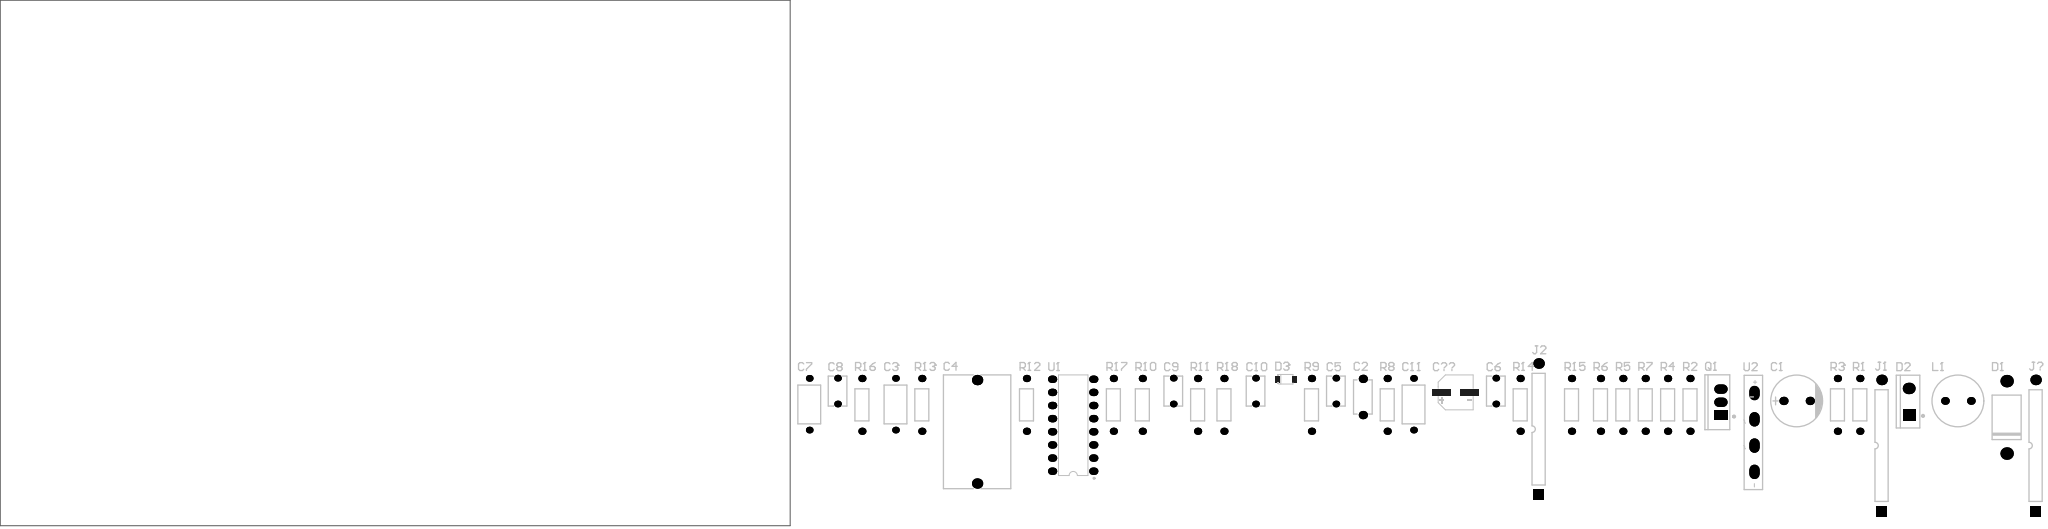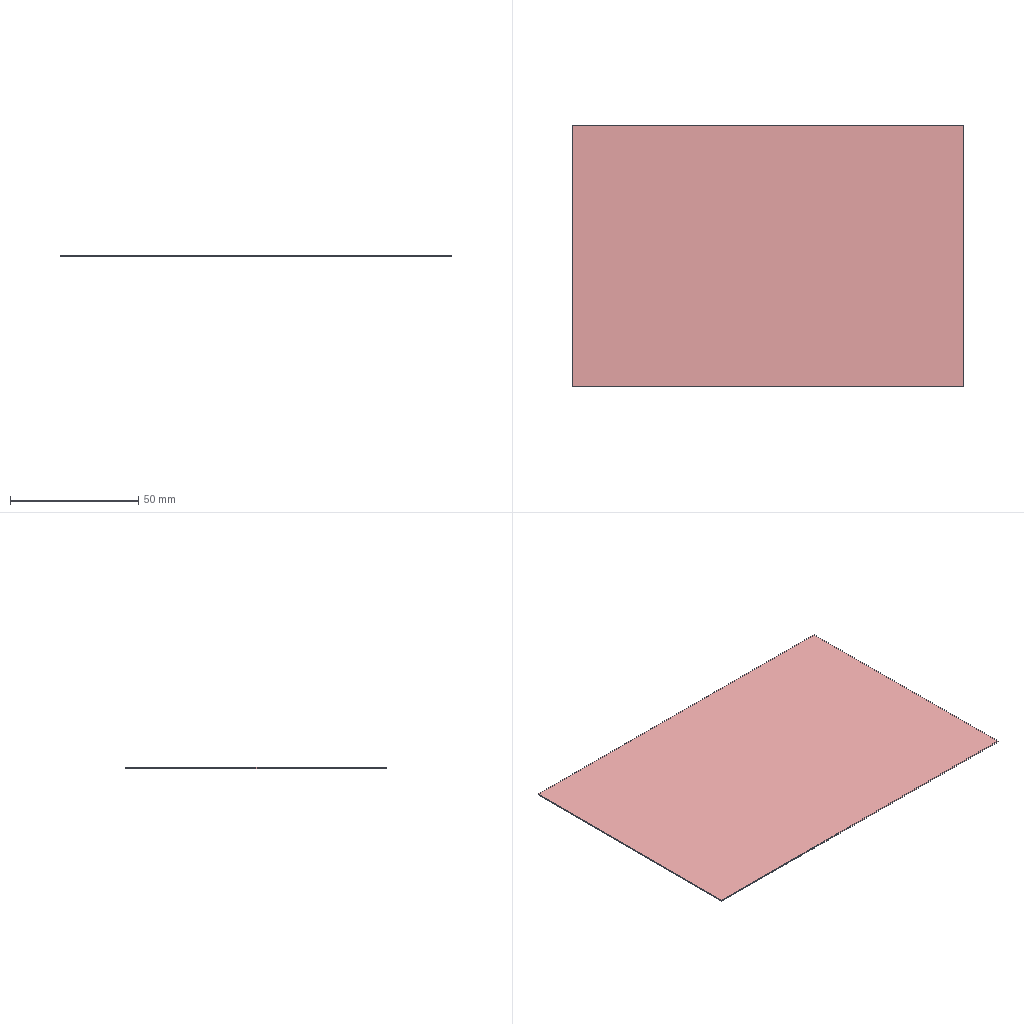Circuit board layout | Altium Designer | box 152.4 x 101.6 x 0.4 mm
Layer stack:
# Altium Designer layer stack of 2 (unit mm; dielectric type: 0 none, 1 core, 2 prepreg, 3 surface material)
index,name,kind,layer,copper_thickness_mm,dielectric_type,dielectric_thickness_mm,dielectric_material,dielectric_constant
0,Top Paste,other,,,,,,
1,Top Overlay,other,,,,,,
2,Top Solder,dielectric,,,3,0.0102,Solder Resist,3.5
3,Top Layer,copper,Top Layer,0.0356,,,,
4,Dielectric 1,dielectric,,,0,0.32,FR-4,4.8
5,Bottom Layer,copper,Bottom Layer,0.0356,,,,
6,Bottom Solder,dielectric,,,3,0.0102,Solder Resist,3.5
7,Bottom Overlay,other,,,,,,
8,Bottom Paste,other,,,,,,
# drill layer pairs: low layer,high layer
drill_pair,Top Layer,Bottom Layer
Part placement:
Designator,Comment,Layer,Footprint,Center-X(mm),Center-Y(mm),Rotation
U2,GBU8K,TopLayer,GBU_4P-L22.0-W3.5-P5.08-GBU4K,363.855,43.434,90
U1,UC3854N,TopLayer,PDIP-16_L19.3-W6.4-P2.54-LS7.94-BL,232.41,44.831,90
R18,MF1/4W-100K±1%-OT26,TopLayer,RES-TH_BD2.7-L6.2-P10.20-D0.4,261.493,48.768,90
R17,MF1/4W-100K±1%-OT26,TopLayer,RES-TH_BD2.7-L6.2-P10.20-D0.4,240.157,48.768,90
R16,MF1/4W-100K±1%-OT26,TopLayer,RES-TH_BD2.7-L6.2-P10.20-D0.4,191.643,48.768,90
R15,MF1/4W-100K±1%-OT26,TopLayer,RES-TH_BD2.7-L6.2-P10.20-D0.4,328.549,48.768,90
R14,MF1/4W-100K±1%-OT26,TopLayer,RES-TH_BD2.7-L6.2-P10.20-D0.4,318.643,48.768,90
R13,MF1/4W-100K±1%-OT26,TopLayer,RES-TH_BD2.7-L6.2-P10.20-D0.4,203.2,48.768,90
R12,MF1/4W-100K±1%-OT26,TopLayer,RES-TH_BD2.7-L6.2-P10.20-D0.4,223.393,48.768,90
R11,MF1/4W-100K±1%-OT26,TopLayer,RES-TH_BD2.7-L6.2-P10.20-D0.4,256.413,48.768,90
R10,MF1/4W-100K±1%-OT26,TopLayer,RES-TH_BD2.7-L6.2-P10.20-D0.4,245.745,48.768,90
R9,MF1/4W-100K±1%-OT26,TopLayer,RES-TH_BD2.7-L6.2-P10.20-D0.4,278.384,48.768,90
R8,MF1/4W-100K±1%-OT26,TopLayer,RES-TH_BD2.7-L6.2-P10.20-D0.4,292.989,48.768,90
R7,MF1/4W-100K±1%-OT26,TopLayer,RES-TH_BD2.7-L6.2-P10.20-D0.4,342.773,48.768,90
R6,MF1/4W-100K±1%-OT26,TopLayer,RES-TH_BD2.7-L6.2-P10.20-D0.4,334.137,48.768,90
R5,MF1/4W-100K±1%-OT26,TopLayer,RES-TH_BD2.7-L6.2-P10.20-D0.4,338.455,48.768,90
R4,MF1/4W-100K±1%-OT26,TopLayer,RES-TH_BD2.7-L6.2-P10.20-D0.4,347.091,48.768,90
R3,MF1/4W-100K±1%-OT26,TopLayer,RES-TH_BD2.7-L6.2-P10.20-D0.4,379.857,48.768,90
R2,MF1/4W-100K±1%-OT26,TopLayer,RES-TH_BD2.7-L6.2-P10.20-D0.4,351.409,48.768,90
R1,MF1/4W-100K±1%-OT26,TopLayer,RES-TH_BD2.7-L6.2-P10.20-D0.4,384.175,48.768,90
Q1,IRF530NPBF,TopLayer,TO-220-3_L10.0-W4.5-P2.54-L,357.378,49.276,90
L1,XR8*10-101K-L,TopLayer,IND-TH_BD10.0-P5.00-D0.6,403.098,49.53,0
J?,HOLE,TopLayer,DIP2,418.084,40.894,90
J2,HOLE,TopLayer,DIP2,322.199,44.069,90
J1,HOLE,TopLayer,DIP2,388.366,40.894,90
D3,BZT52C8V2_C19077406,TopLayer,SOD-123_L2.7-W1.6-LS3.7-RD,273.431,53.721,0
D2,GC3D10060A,TopLayer,TO-220-2_L10.2-W4.5-P5.08-L-A,393.7,49.403,90
D1,1N5406_C5338388,TopLayer,DO-27_BD5.2-L8.9-P12.90-D1.5-RD,412.496,46.355,90
C??,RVE100UF35V67RV0072,TopLayer,CAP-SMD_BD6.3-L6.6-W6.6-LS7.6-FD-1,306.197,51.181,0
C11,KY1102M400VAC70Y10093,TopLayer,CAP-TH_L7.5-W4.5-P10.00-D0.6,298.069,48.895,90
C10,178MU0002,TopLayer,CAP-TH_L5.8-W3.6-P5.0-D0.6,267.589,51.435,90
C9,178MU0002,TopLayer,CAP-TH_L5.8-W3.6-P5.0-D0.6,251.714,51.435,90
C8,178MU0002,TopLayer,CAP-TH_L5.8-W3.6-P5.0-D0.6,186.944,51.435,90
C7,KY1102M400VAC70Y10093,TopLayer,CAP-TH_L7.5-W4.5-P10.00-D0.6,181.483,48.895,90
C6,178MU0002,TopLayer,CAP-TH_L5.8-W3.6-P5.0-D0.6,313.944,51.435,90
C5,178MU0002,TopLayer,CAP-TH_L5.8-W3.6-P5.0-D0.6,283.083,51.435,90
C4,CBB21-400V/255JP20,TopLayer,CAP-TH_L22.0-W12.5-P20.00-D0.7-FD,213.868,43.561,90
C3,KY1102M400VAC70Y10093,TopLayer,CAP-TH_L7.5-W4.5-P10.00-D0.6,198.12,48.895,90
C2,KJKF222M2FF7035A075E,TopLayer,CAP-TH_L6.5-W3.5-P7.50-D1.0,288.29,50.292,90
C1,LKME1402A101MF,TopLayer,CAP-TH_BD10.0-P5.00-D1.0-FD,371.983,49.53,0
Pad and via stacks:
# Altium Designer via and pad stacks of 2 (unit mm). Each distinct definition once, with the count of objects using it.
# via: kind,start_layer,end_layer,hole_mm,diameter_mm,mode(0 simple;1 top-mid-bottom;2 full stack),diameter_per_layer,count,example_net
# pad: kind,layer,hole_mm,hole_type(0 round;1 square;2 slot),plating,top_size,top_shape(1 round;2 rect;3 octagon;9 rounded rect),mid_size,bottom_size,mode,footprint,size_per_layer,count,example
pad,Multi-Layer,1.016,0,plated,2.032x2.032,1,2.032x2.032,2.032x2.032,0,DIP2,,2,J2.2
pad,Multi-Layer,1.016,0,plated,2.032x2.032,2,2.032x2.032,2.032x2.032,0,DIP2,,2,J2.1
pad,Multi-Layer,1.2,0,plated,1.8x2.6,2,1.8x2.6,1.8x2.6,0,TO-220-3_L10.0-W4.5-P2.54-L,,1,Q1.1
pad,Multi-Layer,1.2,0,plated,1.8x2.6,1,1.8x2.6,1.8x2.6,0,TO-220-3_L10.0-W4.5-P2.54-L,,2,Q1.3
pad,Multi-Layer,0.8,0,plated,1.4x1.4,1,1.4x1.4,1.4x1.4,0,RES-TH_BD2.7-L6.2-P10.20-D0.4,,36,R10.2
pad,Multi-Layer,0.8,0,plated,1.3x1.3,1,1.3x1.3,1.3x1.3,0,CAP-TH_L5.8-W3.6-P5.0-D0.6,,10,C9.1
pad,Multi-Layer,0.7,0,plated,1.3x1.3,1,1.3x1.3,1.3x1.3,0,CAP-TH_L7.5-W4.5-P10.00-D0.6,,6,C7.2
pad,Multi-Layer,1.2,0,plated,2x2,1,2x2,2x2,0,CAP-TH_L22.0-W12.5-P20.00-D0.7-FD,,2,C4.1
pad,Multi-Layer,0.8,0,plated,1.44x1.8,1,1.44x1.8,1.44x1.8,0,PDIP-16_L19.3-W6.4-P2.54-LS7.94-BL,,16,U1.9
pad,Multi-Layer,1,0,plated,1.6x1.6,1,1.6x1.6,1.6x1.6,0,CAP-TH_L6.5-W3.5-P7.50-D1.0,,2,C2.2
pad,Multi-Layer,1.2,2,plated,2.8x2,1,2.8x2,2.8x2,0,GBU_4P-L22.0-W3.5-P5.08-GBU4K,,4,U2.4
pad,Multi-Layer,1,0,plated,1.6x1.6,1,1.6x1.6,1.6x1.6,0,CAP-TH_BD10.0-P5.00-D1.0-FD,,2,C1.2
pad,Multi-Layer,1.3,0,plated,2.2x2.5,2,2.2x2.5,2.2x2.5,0,TO-220-2_L10.2-W4.5-P5.08-L-A,,1,D2.1
pad,Multi-Layer,1.3,0,plated,2.2x2.5,1,2.2x2.5,2.2x2.5,0,TO-220-2_L10.2-W4.5-P5.08-L-A,,1,D2.3
pad,Multi-Layer,0.9,0,plated,1.5x1.5,1,1.5x1.5,1.5x1.5,0,IND-TH_BD10.0-P5.00-D0.6,,2,L1.1
pad,Multi-Layer,1.6,0,plated,2.4x2.4,1,2.4x2.4,2.4x2.4,0,DO-27_BD5.2-L8.9-P12.90-D1.5-RD,,2,D1.1
pad,Top Layer,0,0,plated,0.91x1.22,2,0.91x1.22,0.91x1.22,0,SOD-123_L2.7-W1.6-LS3.7-RD,,2,D3.1
pad,Top Layer,0,0,plated,3.5x1.2,2,3.5x1.2,3.5x1.2,0,CAP-SMD_BD6.3-L6.6-W6.6-LS7.6-FD-1,,2,C??.2
Copper pours:
name,layer,net,type(0 solid;1 hatched;2 none)
G,Bottom Layer,GND,0
G,Top Layer,GND,0
Design rules, without the lines most boards share:
# Altium Designer design rules of 2 (exported by Altium Designer, unit mm)
# columns: name | kind | enabled | priority | scope1 | scope2 | descriptor | typed fields (field=value)
Clearance | 0 | enabled | 1 | All | All | Clearance Constraint (Gap=10mil) (All),(All) | gap=0.254
PlaneConnect | 6 | enabled | 1 | All | All | Power Plane Connect Rule(Relief Connect )(Expansion=20mil) (Conductor Width=10mil) (Air Gap=10mil) (Entries=4) (All) | relief_conductor_width=0.254 relief_entries=4 relief_expansion=0.508
PolygonConnect | 20 | enabled | 1 | All | All | Polygon Connect Rule(Relief Connect )(Conductor Width=10mil) (Relief Angle=90 Angle) (Entries=4) (Air Gap Width=10mil) (All),(All) | connect_style(0=relief,1=direct,2=none)=0 relief_conductor_width=0.254 relief_entries=4
Width | 2 | enabled | 1 | All | All | Width Constraint (Min=10mil) (Max=30mil) (Preferred=10mil) (All) |
RoutingVias | 11 | enabled | 1 | All | All | Routing Via (MinHoleWidth=28mil) (MaxHoleWidth=28mil) (PreferredHoleWidth=28mil) (MinWidth=50mil) (MaxWidth=50mil) (PreferedWidth=50mil) (All) | via_min_hole=0.7112 via_max_hole=0.7112 via_preferred_diameter=1.27 via_preferred_hole=0.7112
PasteMaskExpansion | 14 | enabled | 1 | All | All | Paste Mask Expansion (Expansion =0mil) (All) | expansion=0
SolderMaskExpansion | 13 | enabled | 1 | All | All | Solder Mask Expansion (Expansion =4mil) (All) | expansion=0.1016
DiffPairsRouting | 51 | enabled | 1 | All | All | Differential Pairs Uncoupled Length using the Gap Constraints (Min=10mil) (Max=10mil) (Prefered=10mil)  and Width Constraints (Min=15mil) (Max=15mil) (Prefered=15mil) (All) |
HoleToHoleClearance | 52 | enabled | 1 | All | All | Hole To Hole Clearance (Gap=10mil) (All),(All) | gap=0.254
MinimumSolderMaskSliver | 53 | enabled | 1 | All | All | Minimum Solder Mask Sliver (Gap=0mil) (All),(All) |
SilkToSolderMaskClearance | 54 | enabled | 1 | IsPad | All | Silk To Solder Mask (Clearance=0mil) (IsPad),(All) |
SilkToSilkClearance | 55 | enabled | 1 | All | All | Silk to Silk (Clearance=0mil) (All),(All) |
Classes set for this board:
# Altium Designer classes of 2 (member kind: 0 net, 1 component, 2 from-to, 3 pad, 4 layer, 5 differential pair, 6 design channel, 7 polygon, 8 structure, 9 xSignal)
# columns: class name | member kind | superclass | members
uc3854 | 1 | no | C1; C2; C3; C4; C5; C6; C7; C8; C9; C10; C11; C??; D1; D2; D3; J1; J2; L1; Q1; R1; R2; R3; R4; R5; R6; R7; R8; R9; R10; R11; R12; R13; R14; R15; R16; R17; R18; U1; U2;